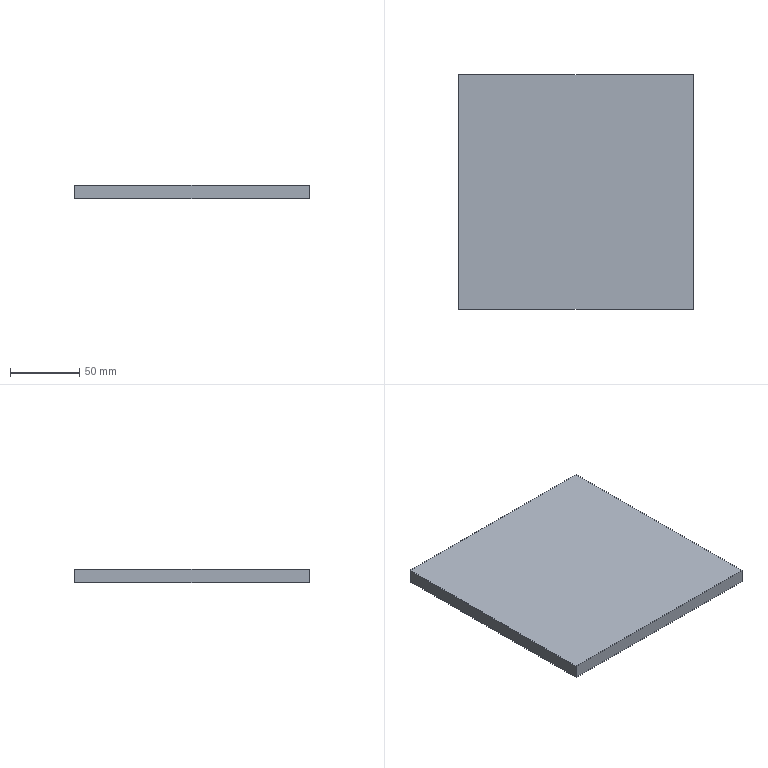Part | STEP file | Motor adjusting plate QY-2-01 | 1 solid | 6 faces | box 170 x 170 x 10 mm | volume 289000 mm3 | plane 6
STEP:
#1=CARTESIAN_POINT('',(0.,0.,0.));
#2=DIRECTION('',(0.,0.,1.));
#3=DIRECTION('',(1.,0.,0.));
#4=AXIS2_PLACEMENT_3D('',#1,#2,#3);
#5=CARTESIAN_POINT('',(85.,-85.,0.));
#6=VERTEX_POINT('',#5);
#7=CARTESIAN_POINT('',(85.,85.,0.));
#8=VERTEX_POINT('',#7);
#9=CARTESIAN_POINT('',(85.,85.,0.));
#10=DIRECTION('',(0.,1.,0.));
#11=VECTOR('',#10,1.);
#12=LINE('',#9,#11);
#13=CARTESIAN_POINT('',(85.,85.,10.));
#14=DIRECTION('',(-1.,0.,0.));
#15=DIRECTION('',(0.,-1.,0.));
#16=AXIS2_PLACEMENT_3D('',#13,#14,#15);
#17=PLANE('',#16);
#18=CARTESIAN_POINT('',(0.,-10.));
#19=DIRECTION('',(-1.,0.));
#20=VECTOR('',#19,1.);
#21=LINE('',#18,#20);
#22=(GEOMETRIC_REPRESENTATION_CONTEXT(2)PARAMETRIC_REPRESENTATION_CONTEXT()REPRESENTATION_CONTEXT('',''));
#23=DEFINITIONAL_REPRESENTATION('',(#21),#22);
#24=PCURVE('',#17,#23);
#25=CARTESIAN_POINT('',(0.,0.,0.));
#26=DIRECTION('',(0.,0.,1.));
#27=DIRECTION('',(1.,0.,0.));
#28=AXIS2_PLACEMENT_3D('',#25,#26,#27);
#29=PLANE('',#28);
#30=CARTESIAN_POINT('',(85.,85.));
#31=DIRECTION('',(0.,1.));
#32=VECTOR('',#31,1.);
#33=LINE('',#30,#32);
#34=(GEOMETRIC_REPRESENTATION_CONTEXT(2)PARAMETRIC_REPRESENTATION_CONTEXT()REPRESENTATION_CONTEXT('',''));
#35=DEFINITIONAL_REPRESENTATION('',(#33),#34);
#36=PCURVE('',#29,#35);
#37=SURFACE_CURVE('',#12,(#24,#36),.PCURVE_S1.);
#38=EDGE_CURVE('',#6,#8,#37,.T.);
#39=ORIENTED_EDGE('',*,*,#38,.T.);
#40=CARTESIAN_POINT('',(85.,85.,10.));
#41=VERTEX_POINT('',#40);
#42=CARTESIAN_POINT('',(85.,85.,10.));
#43=DIRECTION('',(0.,0.,-1.));
#44=VECTOR('',#43,1.);
#45=LINE('',#42,#44);
#46=CARTESIAN_POINT('',(0.,0.));
#47=DIRECTION('',(0.,-1.));
#48=VECTOR('',#47,1.);
#49=LINE('',#46,#48);
#50=(GEOMETRIC_REPRESENTATION_CONTEXT(2)PARAMETRIC_REPRESENTATION_CONTEXT()REPRESENTATION_CONTEXT('',''));
#51=DEFINITIONAL_REPRESENTATION('',(#49),#50);
#52=PCURVE('',#17,#51);
#53=CARTESIAN_POINT('',(-85.,85.,10.));
#54=DIRECTION('',(0.,-1.,0.));
#55=DIRECTION('',(0.,0.,-1.));
#56=AXIS2_PLACEMENT_3D('',#53,#54,#55);
#57=PLANE('',#56);
#58=CARTESIAN_POINT('',(0.,170.));
#59=DIRECTION('',(1.,0.));
#60=VECTOR('',#59,1.);
#61=LINE('',#58,#60);
#62=(GEOMETRIC_REPRESENTATION_CONTEXT(2)PARAMETRIC_REPRESENTATION_CONTEXT()REPRESENTATION_CONTEXT('',''));
#63=DEFINITIONAL_REPRESENTATION('',(#61),#62);
#64=PCURVE('',#57,#63);
#65=SURFACE_CURVE('',#45,(#52,#64),.PCURVE_S1.);
#66=EDGE_CURVE('',#41,#8,#65,.T.);
#67=ORIENTED_EDGE('',*,*,#66,.F.);
#68=CARTESIAN_POINT('',(85.,-85.,10.));
#69=VERTEX_POINT('',#68);
#70=CARTESIAN_POINT('',(85.,85.,10.));
#71=DIRECTION('',(0.,1.,0.));
#72=VECTOR('',#71,1.);
#73=LINE('',#70,#72);
#74=CARTESIAN_POINT('',(0.,0.));
#75=DIRECTION('',(-1.,0.));
#76=VECTOR('',#75,1.);
#77=LINE('',#74,#76);
#78=(GEOMETRIC_REPRESENTATION_CONTEXT(2)PARAMETRIC_REPRESENTATION_CONTEXT()REPRESENTATION_CONTEXT('',''));
#79=DEFINITIONAL_REPRESENTATION('',(#77),#78);
#80=PCURVE('',#17,#79);
#81=CARTESIAN_POINT('',(0.,0.,10.));
#82=DIRECTION('',(0.,0.,1.));
#83=DIRECTION('',(1.,0.,0.));
#84=AXIS2_PLACEMENT_3D('',#81,#82,#83);
#85=PLANE('',#84);
#86=CARTESIAN_POINT('',(85.,85.));
#87=DIRECTION('',(0.,1.));
#88=VECTOR('',#87,1.);
#89=LINE('',#86,#88);
#90=(GEOMETRIC_REPRESENTATION_CONTEXT(2)PARAMETRIC_REPRESENTATION_CONTEXT()REPRESENTATION_CONTEXT('',''));
#91=DEFINITIONAL_REPRESENTATION('',(#89),#90);
#92=PCURVE('',#85,#91);
#93=SURFACE_CURVE('',#73,(#80,#92),.PCURVE_S1.);
#94=EDGE_CURVE('',#69,#41,#93,.T.);
#95=ORIENTED_EDGE('',*,*,#94,.F.);
#96=CARTESIAN_POINT('',(85.,-85.,10.));
#97=DIRECTION('',(0.,0.,-1.));
#98=VECTOR('',#97,1.);
#99=LINE('',#96,#98);
#100=CARTESIAN_POINT('',(170.,0.));
#101=DIRECTION('',(0.,-1.));
#102=VECTOR('',#101,1.);
#103=LINE('',#100,#102);
#104=(GEOMETRIC_REPRESENTATION_CONTEXT(2)PARAMETRIC_REPRESENTATION_CONTEXT()REPRESENTATION_CONTEXT('',''));
#105=DEFINITIONAL_REPRESENTATION('',(#103),#104);
#106=PCURVE('',#17,#105);
#107=CARTESIAN_POINT('',(-85.,-85.,10.));
#108=DIRECTION('',(0.,1.,0.));
#109=DIRECTION('',(0.,0.,1.));
#110=AXIS2_PLACEMENT_3D('',#107,#108,#109);
#111=PLANE('',#110);
#112=CARTESIAN_POINT('',(0.,170.));
#113=DIRECTION('',(-1.,0.));
#114=VECTOR('',#113,1.);
#115=LINE('',#112,#114);
#116=(GEOMETRIC_REPRESENTATION_CONTEXT(2)PARAMETRIC_REPRESENTATION_CONTEXT()REPRESENTATION_CONTEXT('',''));
#117=DEFINITIONAL_REPRESENTATION('',(#115),#116);
#118=PCURVE('',#111,#117);
#119=SURFACE_CURVE('',#99,(#106,#118),.PCURVE_S1.);
#120=EDGE_CURVE('',#69,#6,#119,.T.);
#121=ORIENTED_EDGE('',*,*,#120,.T.);
#122=EDGE_LOOP('',(#39,#67,#95,#121));
#123=FACE_BOUND('',#122,.T.);
#124=ADVANCED_FACE('',(#123),#17,.F.);
#125=CARTESIAN_POINT('',(-85.,85.,0.));
#126=VERTEX_POINT('',#125);
#127=CARTESIAN_POINT('',(-85.,85.,0.));
#128=DIRECTION('',(-1.,0.,0.));
#129=VECTOR('',#128,1.);
#130=LINE('',#127,#129);
#131=CARTESIAN_POINT('',(10.,0.));
#132=DIRECTION('',(0.,-1.));
#133=VECTOR('',#132,1.);
#134=LINE('',#131,#133);
#135=(GEOMETRIC_REPRESENTATION_CONTEXT(2)PARAMETRIC_REPRESENTATION_CONTEXT()REPRESENTATION_CONTEXT('',''));
#136=DEFINITIONAL_REPRESENTATION('',(#134),#135);
#137=PCURVE('',#57,#136);
#138=CARTESIAN_POINT('',(-85.,85.));
#139=DIRECTION('',(-1.,0.));
#140=VECTOR('',#139,1.);
#141=LINE('',#138,#140);
#142=(GEOMETRIC_REPRESENTATION_CONTEXT(2)PARAMETRIC_REPRESENTATION_CONTEXT()REPRESENTATION_CONTEXT('',''));
#143=DEFINITIONAL_REPRESENTATION('',(#141),#142);
#144=PCURVE('',#29,#143);
#145=SURFACE_CURVE('',#130,(#137,#144),.PCURVE_S1.);
#146=EDGE_CURVE('',#8,#126,#145,.T.);
#147=ORIENTED_EDGE('',*,*,#146,.T.);
#148=CARTESIAN_POINT('',(-85.,85.,10.));
#149=VERTEX_POINT('',#148);
#150=CARTESIAN_POINT('',(-85.,85.,10.));
#151=DIRECTION('',(0.,0.,-1.));
#152=VECTOR('',#151,1.);
#153=LINE('',#150,#152);
#154=CARTESIAN_POINT('',(0.,0.));
#155=DIRECTION('',(1.,0.));
#156=VECTOR('',#155,1.);
#157=LINE('',#154,#156);
#158=(GEOMETRIC_REPRESENTATION_CONTEXT(2)PARAMETRIC_REPRESENTATION_CONTEXT()REPRESENTATION_CONTEXT('',''));
#159=DEFINITIONAL_REPRESENTATION('',(#157),#158);
#160=PCURVE('',#57,#159);
#161=CARTESIAN_POINT('',(-85.,85.,10.));
#162=DIRECTION('',(1.,0.,0.));
#163=DIRECTION('',(0.,1.,0.));
#164=AXIS2_PLACEMENT_3D('',#161,#162,#163);
#165=PLANE('',#164);
#166=CARTESIAN_POINT('',(0.,0.));
#167=DIRECTION('',(0.,-1.));
#168=VECTOR('',#167,1.);
#169=LINE('',#166,#168);
#170=(GEOMETRIC_REPRESENTATION_CONTEXT(2)PARAMETRIC_REPRESENTATION_CONTEXT()REPRESENTATION_CONTEXT('',''));
#171=DEFINITIONAL_REPRESENTATION('',(#169),#170);
#172=PCURVE('',#165,#171);
#173=SURFACE_CURVE('',#153,(#160,#172),.PCURVE_S1.);
#174=EDGE_CURVE('',#149,#126,#173,.T.);
#175=ORIENTED_EDGE('',*,*,#174,.F.);
#176=CARTESIAN_POINT('',(-85.,85.,10.));
#177=DIRECTION('',(-1.,0.,0.));
#178=VECTOR('',#177,1.);
#179=LINE('',#176,#178);
#180=CARTESIAN_POINT('',(0.,0.));
#181=DIRECTION('',(0.,-1.));
#182=VECTOR('',#181,1.);
#183=LINE('',#180,#182);
#184=(GEOMETRIC_REPRESENTATION_CONTEXT(2)PARAMETRIC_REPRESENTATION_CONTEXT()REPRESENTATION_CONTEXT('',''));
#185=DEFINITIONAL_REPRESENTATION('',(#183),#184);
#186=PCURVE('',#57,#185);
#187=CARTESIAN_POINT('',(-85.,85.));
#188=DIRECTION('',(-1.,0.));
#189=VECTOR('',#188,1.);
#190=LINE('',#187,#189);
#191=(GEOMETRIC_REPRESENTATION_CONTEXT(2)PARAMETRIC_REPRESENTATION_CONTEXT()REPRESENTATION_CONTEXT('',''));
#192=DEFINITIONAL_REPRESENTATION('',(#190),#191);
#193=PCURVE('',#85,#192);
#194=SURFACE_CURVE('',#179,(#186,#193),.PCURVE_S1.);
#195=EDGE_CURVE('',#41,#149,#194,.T.);
#196=ORIENTED_EDGE('',*,*,#195,.F.);
#197=ORIENTED_EDGE('',*,*,#66,.T.);
#198=EDGE_LOOP('',(#147,#175,#196,#197));
#199=FACE_BOUND('',#198,.T.);
#200=ADVANCED_FACE('',(#199),#57,.F.);
#201=CARTESIAN_POINT('',(-85.,-85.,0.));
#202=VERTEX_POINT('',#201);
#203=CARTESIAN_POINT('',(-85.,85.,0.));
#204=DIRECTION('',(0.,-1.,0.));
#205=VECTOR('',#204,1.);
#206=LINE('',#203,#205);
#207=CARTESIAN_POINT('',(0.,-10.));
#208=DIRECTION('',(-1.,0.));
#209=VECTOR('',#208,1.);
#210=LINE('',#207,#209);
#211=(GEOMETRIC_REPRESENTATION_CONTEXT(2)PARAMETRIC_REPRESENTATION_CONTEXT()REPRESENTATION_CONTEXT('',''));
#212=DEFINITIONAL_REPRESENTATION('',(#210),#211);
#213=PCURVE('',#165,#212);
#214=CARTESIAN_POINT('',(-85.,85.));
#215=DIRECTION('',(0.,-1.));
#216=VECTOR('',#215,1.);
#217=LINE('',#214,#216);
#218=(GEOMETRIC_REPRESENTATION_CONTEXT(2)PARAMETRIC_REPRESENTATION_CONTEXT()REPRESENTATION_CONTEXT('',''));
#219=DEFINITIONAL_REPRESENTATION('',(#217),#218);
#220=PCURVE('',#29,#219);
#221=SURFACE_CURVE('',#206,(#213,#220),.PCURVE_S1.);
#222=EDGE_CURVE('',#126,#202,#221,.T.);
#223=ORIENTED_EDGE('',*,*,#222,.T.);
#224=CARTESIAN_POINT('',(-85.,-85.,10.));
#225=VERTEX_POINT('',#224);
#226=CARTESIAN_POINT('',(-85.,-85.,10.));
#227=DIRECTION('',(0.,0.,-1.));
#228=VECTOR('',#227,1.);
#229=LINE('',#226,#228);
#230=CARTESIAN_POINT('',(-170.,0.));
#231=DIRECTION('',(0.,-1.));
#232=VECTOR('',#231,1.);
#233=LINE('',#230,#232);
#234=(GEOMETRIC_REPRESENTATION_CONTEXT(2)PARAMETRIC_REPRESENTATION_CONTEXT()REPRESENTATION_CONTEXT('',''));
#235=DEFINITIONAL_REPRESENTATION('',(#233),#234);
#236=PCURVE('',#165,#235);
#237=CARTESIAN_POINT('',(0.,0.));
#238=DIRECTION('',(-1.,0.));
#239=VECTOR('',#238,1.);
#240=LINE('',#237,#239);
#241=(GEOMETRIC_REPRESENTATION_CONTEXT(2)PARAMETRIC_REPRESENTATION_CONTEXT()REPRESENTATION_CONTEXT('',''));
#242=DEFINITIONAL_REPRESENTATION('',(#240),#241);
#243=PCURVE('',#111,#242);
#244=SURFACE_CURVE('',#229,(#236,#243),.PCURVE_S1.);
#245=EDGE_CURVE('',#225,#202,#244,.T.);
#246=ORIENTED_EDGE('',*,*,#245,.F.);
#247=CARTESIAN_POINT('',(-85.,85.,10.));
#248=DIRECTION('',(0.,-1.,0.));
#249=VECTOR('',#248,1.);
#250=LINE('',#247,#249);
#251=CARTESIAN_POINT('',(0.,0.));
#252=DIRECTION('',(-1.,0.));
#253=VECTOR('',#252,1.);
#254=LINE('',#251,#253);
#255=(GEOMETRIC_REPRESENTATION_CONTEXT(2)PARAMETRIC_REPRESENTATION_CONTEXT()REPRESENTATION_CONTEXT('',''));
#256=DEFINITIONAL_REPRESENTATION('',(#254),#255);
#257=PCURVE('',#165,#256);
#258=CARTESIAN_POINT('',(-85.,85.));
#259=DIRECTION('',(0.,-1.));
#260=VECTOR('',#259,1.);
#261=LINE('',#258,#260);
#262=(GEOMETRIC_REPRESENTATION_CONTEXT(2)PARAMETRIC_REPRESENTATION_CONTEXT()REPRESENTATION_CONTEXT('',''));
#263=DEFINITIONAL_REPRESENTATION('',(#261),#262);
#264=PCURVE('',#85,#263);
#265=SURFACE_CURVE('',#250,(#257,#264),.PCURVE_S1.);
#266=EDGE_CURVE('',#149,#225,#265,.T.);
#267=ORIENTED_EDGE('',*,*,#266,.F.);
#268=ORIENTED_EDGE('',*,*,#174,.T.);
#269=EDGE_LOOP('',(#223,#246,#267,#268));
#270=FACE_BOUND('',#269,.T.);
#271=ADVANCED_FACE('',(#270),#165,.F.);
#272=CARTESIAN_POINT('',(-85.,-85.,0.));
#273=DIRECTION('',(1.,0.,0.));
#274=VECTOR('',#273,1.);
#275=LINE('',#272,#274);
#276=CARTESIAN_POINT('',(-10.,0.));
#277=DIRECTION('',(0.,1.));
#278=VECTOR('',#277,1.);
#279=LINE('',#276,#278);
#280=(GEOMETRIC_REPRESENTATION_CONTEXT(2)PARAMETRIC_REPRESENTATION_CONTEXT()REPRESENTATION_CONTEXT('',''));
#281=DEFINITIONAL_REPRESENTATION('',(#279),#280);
#282=PCURVE('',#111,#281);
#283=CARTESIAN_POINT('',(-85.,-85.));
#284=DIRECTION('',(1.,0.));
#285=VECTOR('',#284,1.);
#286=LINE('',#283,#285);
#287=(GEOMETRIC_REPRESENTATION_CONTEXT(2)PARAMETRIC_REPRESENTATION_CONTEXT()REPRESENTATION_CONTEXT('',''));
#288=DEFINITIONAL_REPRESENTATION('',(#286),#287);
#289=PCURVE('',#29,#288);
#290=SURFACE_CURVE('',#275,(#282,#289),.PCURVE_S1.);
#291=EDGE_CURVE('',#202,#6,#290,.T.);
#292=ORIENTED_EDGE('',*,*,#291,.T.);
#293=ORIENTED_EDGE('',*,*,#120,.F.);
#294=CARTESIAN_POINT('',(-85.,-85.,10.));
#295=DIRECTION('',(1.,0.,0.));
#296=VECTOR('',#295,1.);
#297=LINE('',#294,#296);
#298=CARTESIAN_POINT('',(0.,0.));
#299=DIRECTION('',(0.,1.));
#300=VECTOR('',#299,1.);
#301=LINE('',#298,#300);
#302=(GEOMETRIC_REPRESENTATION_CONTEXT(2)PARAMETRIC_REPRESENTATION_CONTEXT()REPRESENTATION_CONTEXT('',''));
#303=DEFINITIONAL_REPRESENTATION('',(#301),#302);
#304=PCURVE('',#111,#303);
#305=CARTESIAN_POINT('',(-85.,-85.));
#306=DIRECTION('',(1.,0.));
#307=VECTOR('',#306,1.);
#308=LINE('',#305,#307);
#309=(GEOMETRIC_REPRESENTATION_CONTEXT(2)PARAMETRIC_REPRESENTATION_CONTEXT()REPRESENTATION_CONTEXT('',''));
#310=DEFINITIONAL_REPRESENTATION('',(#308),#309);
#311=PCURVE('',#85,#310);
#312=SURFACE_CURVE('',#297,(#304,#311),.PCURVE_S1.);
#313=EDGE_CURVE('',#225,#69,#312,.T.);
#314=ORIENTED_EDGE('',*,*,#313,.F.);
#315=ORIENTED_EDGE('',*,*,#245,.T.);
#316=EDGE_LOOP('',(#292,#293,#314,#315));
#317=FACE_BOUND('',#316,.T.);
#318=ADVANCED_FACE('',(#317),#111,.F.);
#319=ORIENTED_EDGE('',*,*,#94,.T.);
#320=ORIENTED_EDGE('',*,*,#195,.T.);
#321=ORIENTED_EDGE('',*,*,#266,.T.);
#322=ORIENTED_EDGE('',*,*,#313,.T.);
#323=EDGE_LOOP('',(#319,#320,#321,#322));
#324=FACE_BOUND('',#323,.T.);
#325=ADVANCED_FACE('',(#324),#85,.T.);
#326=ORIENTED_EDGE('',*,*,#38,.F.);
#327=ORIENTED_EDGE('',*,*,#291,.F.);
#328=ORIENTED_EDGE('',*,*,#222,.F.);
#329=ORIENTED_EDGE('',*,*,#146,.F.);
#330=EDGE_LOOP('',(#326,#327,#328,#329));
#331=FACE_BOUND('',#330,.T.);
#332=ADVANCED_FACE('',(#331),#29,.F.);
#333=CLOSED_SHELL('',(#124,#200,#271,#318,#325,#332));
#334=MANIFOLD_SOLID_BREP('',#333);
#335=(LENGTH_UNIT()NAMED_UNIT(*)SI_UNIT(.MILLI.,.METRE.));
#336=UNCERTAINTY_MEASURE_WITH_UNIT(LENGTH_MEASURE(0.0000001),#335,'','');
#337=(NAMED_UNIT(*)PLANE_ANGLE_UNIT()SI_UNIT($,.RADIAN.));
#338=(NAMED_UNIT(*)SI_UNIT($,.STERADIAN.)SOLID_ANGLE_UNIT());
#339=(GEOMETRIC_REPRESENTATION_CONTEXT(3)GLOBAL_UNCERTAINTY_ASSIGNED_CONTEXT((#336))GLOBAL_UNIT_ASSIGNED_CONTEXT((#335,#337,#338))REPRESENTATION_CONTEXT('',''));
#340=ADVANCED_BREP_SHAPE_REPRESENTATION('',(#4,#334),#339);